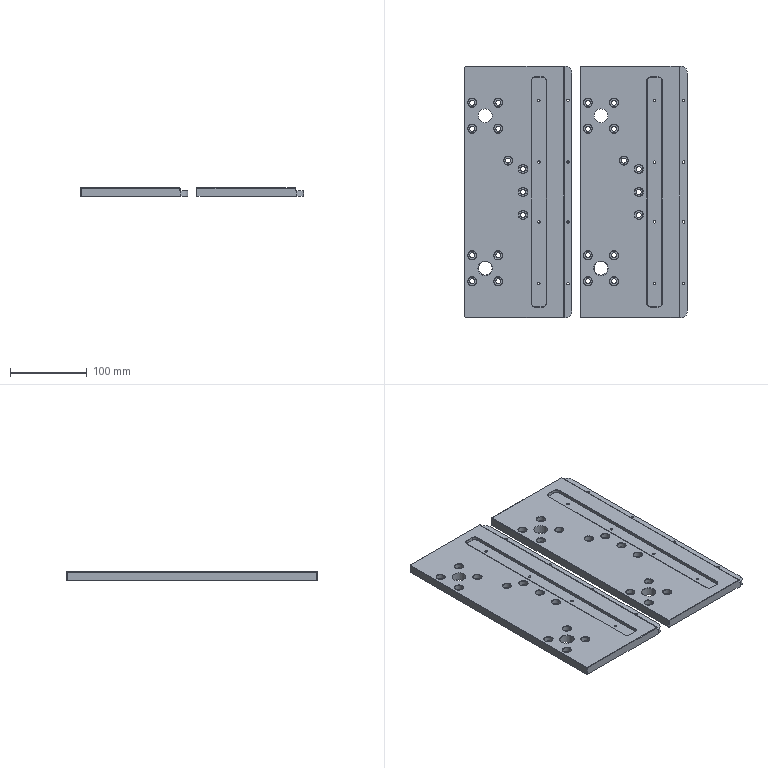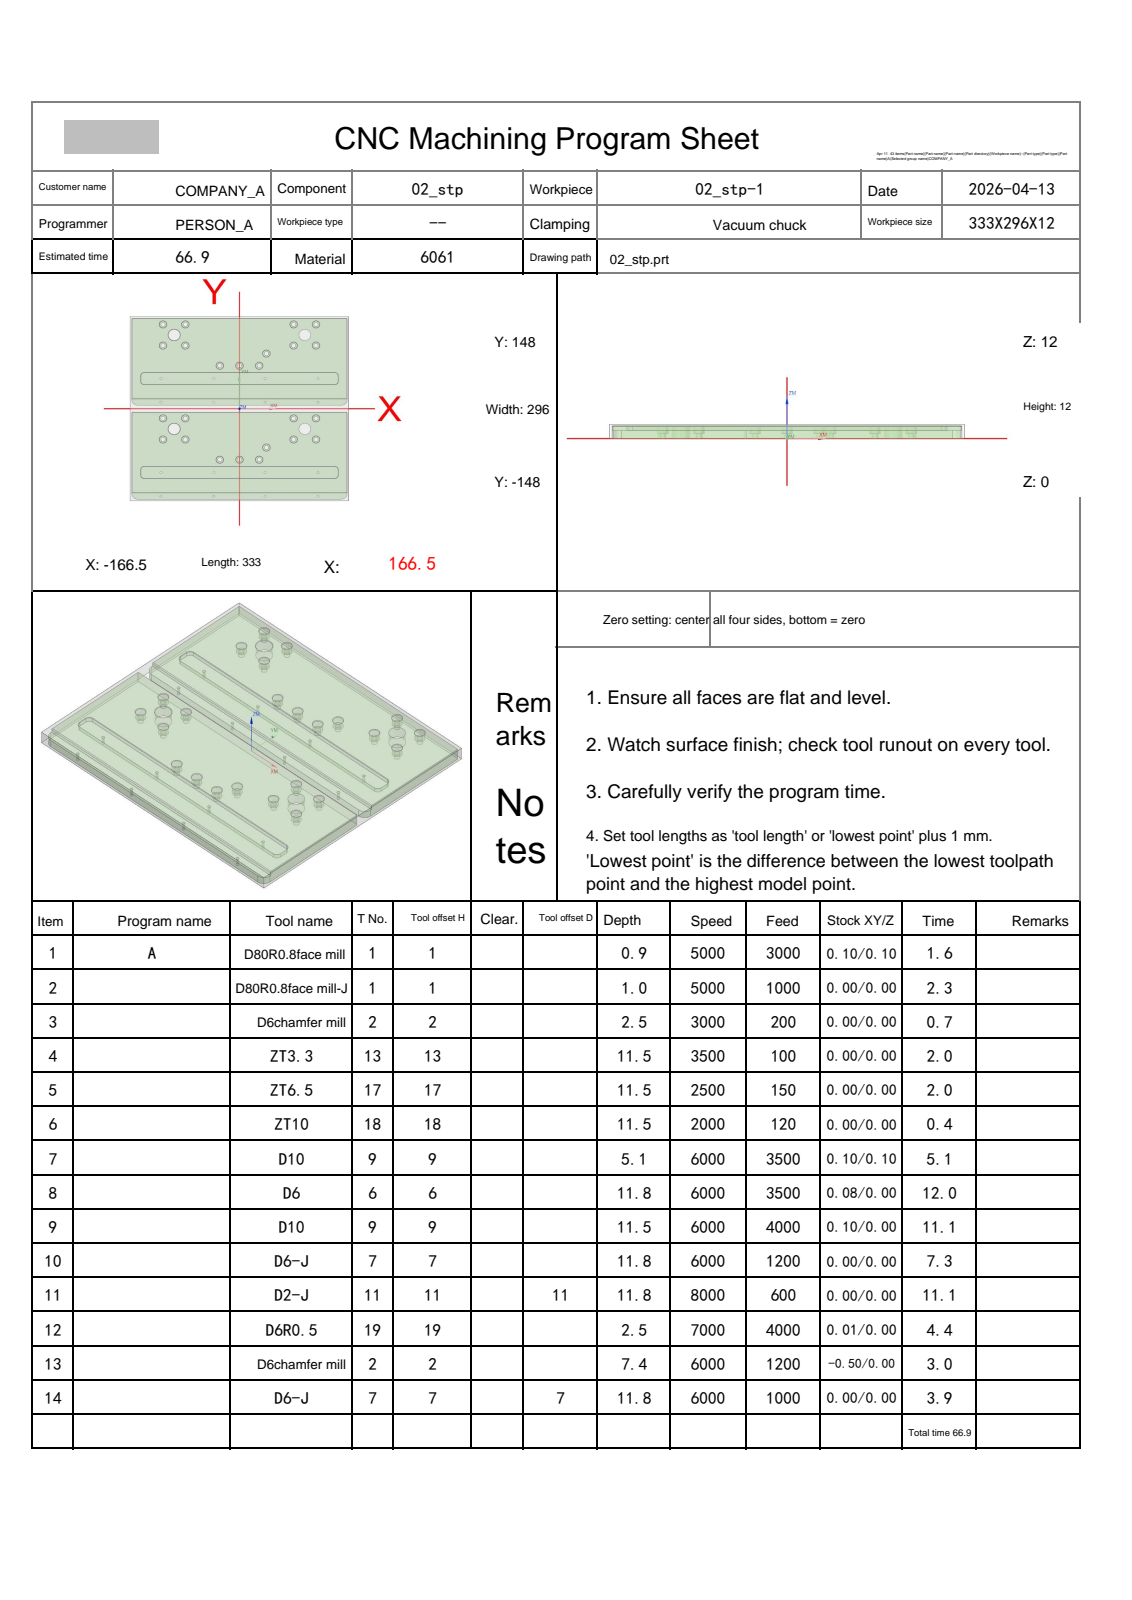NC program | NX | posted by the shop | part box 291 x 328 x 11 mm
Lines 3920 to 4804 of 9762:
N11 T11 M06
(D2-J  D=2. R=0. H=11 ce=0.00 di=0.00)
G00 G90 G54 X80.455 Y134.651 M03 S8000
G43 H11 Z31.
M08
Z5.
G01 X80.479 Y134.582 Z4.996 F600.
X80.675 Y134.236 Z4.975
X80.93 Y133.93 Z4.954
X81.236 Y133.675 Z4.934
X81.582 Y133.479 Z4.913
X81.958 Y133.347 Z4.892
X82.351 Y133.285 Z4.871
X82.649 Z4.855
X83.042 Y133.347 Z4.835
X83.418 Y133.479 Z4.814
X83.764 Y133.675 Z4.793
X84.07 Y133.93 Z4.772
X84.325 Y134.236 Z4.751
X84.521 Y134.582 Z4.73
X84.653 Y134.958 Z4.709
X84.715 Y135.351 Z4.688
Y135.649 Z4.673
X84.654 Y136.038 Z4.652
X84.525 Y136.41 Z4.632
X84.332 Y136.753 Z4.611
X84.082 Y137.057 Z4.59
X83.782 Y137.312 Z4.57
X83.442 Y137.51 Z4.549
X83.072 Y137.645 Z4.528
X82.684 Y137.712 Z4.508
X82.535 Y137.715 Z4.5
G41 D11
X82.5 Y137.75
G03 X80.25 Y135.5 Z4.417 I0.0 J-2.25
X82.5 Y133.25 Z4.335 I2.25 J0.0
X84.75 Y135.5 Z4.252 I0.0 J2.25
X82.5 Y137.75 Z4.169 I-2.25 J0.0
X80.25 Y135.5 Z4.087 I0.0 J-2.25
X82.5 Y133.25 Z4.004 I2.25 J0.0
X84.75 Y135.5 Z3.921 I0.0 J2.25
X82.5 Y137.75 Z3.838 I-2.25 J0.0
X80.25 Y135.5 Z3.756 I0.0 J-2.25
X82.5 Y133.25 Z3.673 I2.25 J0.0
X84.75 Y135.5 Z3.59 I0.0 J2.25
X82.5 Y137.75 Z3.508 I-2.25 J0.0
X80.25 Y135.5 Z3.425 I0.0 J-2.25
X82.5 Y133.25 Z3.342 I2.25 J0.0
X84.75 Y135.5 Z3.26 I0.0 J2.25
X82.5 Y137.75 Z3.177 I-2.25 J0.0
X80.25 Y135.5 Z3.094 I0.0 J-2.25
X82.5 Y133.25 Z3.012 I2.25 J0.0
X84.75 Y135.5 Z2.929 I0.0 J2.25
X82.5 Y137.75 Z2.846 I-2.25 J0.0
X80.25 Y135.5 Z2.763 I0.0 J-2.25
X82.5 Y133.25 Z2.681 I2.25 J0.0
X84.75 Y135.5 Z2.598 I0.0 J2.25
X82.5 Y137.75 Z2.515 I-2.25 J0.0
X80.25 Y135.5 Z2.433 I0.0 J-2.25
X82.5 Y133.25 Z2.35 I2.25 J0.0
X84.75 Y135.5 Z2.267 I0.0 J2.25
X82.5 Y137.75 Z2.185 I-2.25 J0.0
X80.25 Y135.5 Z2.102 I0.0 J-2.25
X82.5 Y133.25 Z2.019 I2.25 J0.0
X84.75 Y135.5 Z1.937 I0.0 J2.25
X82.5 Y137.75 Z1.854 I-2.25 J0.0
X80.25 Y135.5 Z1.771 I0.0 J-2.25
X82.5 Y133.25 Z1.688 I2.25 J0.0
X84.75 Y135.5 Z1.606 I0.0 J2.25
X82.5 Y137.75 Z1.523 I-2.25 J0.0
X80.25 Y135.5 Z1.44 I0.0 J-2.25
X82.5 Y133.25 Z1.358 I2.25 J0.0
X84.75 Y135.5 Z1.275 I0.0 J2.25
X82.5 Y137.75 Z1.192 I-2.25 J0.0
X80.25 Y135.5 Z1.11 I0.0 J-2.25
X82.5 Y133.25 Z1.027 I2.25 J0.0
X84.75 Y135.5 Z.944 I0.0 J2.25
X82.5 Y137.75 Z.862 I-2.25 J0.0
X80.25 Y135.5 Z.779 I0.0 J-2.25
X82.5 Y133.25 Z.696 I2.25 J0.0
X84.75 Y135.5 Z.613 I0.0 J2.25
X82.5 Y137.75 Z.531 I-2.25 J0.0
X80.25 Y135.5 Z.448 I0.0 J-2.25
X82.5 Y133.25 Z.365 I2.25 J0.0
X84.75 Y135.5 Z.283 I0.0 J2.25
X82.5 Y137.75 Z.2 I-2.25 J0.0
X80.25 Y135.5 I0.0 J-2.25
X82.5 Y133.25 I2.25 J0.0
X84.75 Y135.5 I0.0 J2.25
X82.5 Y137.75 I-2.25 J0.0
X82.102 Y137.715 I0.0 J-2.25
G01 X82.075 Y137.707
X82.059 Y137.684
X82.062 Y137.656
G40 X82.071 Y137.607
Z1.2
G00 Z31.
X114.455 Y134.651
Z5.
G01 X114.479 Y134.582 Z4.996
X114.675 Y134.236 Z4.975
X114.93 Y133.93 Z4.954
X115.236 Y133.675 Z4.934
X115.582 Y133.479 Z4.913
X115.958 Y133.347 Z4.892
X116.351 Y133.285 Z4.871
X116.649 Z4.855
X117.042 Y133.347 Z4.835
X117.418 Y133.479 Z4.814
X117.764 Y133.675 Z4.793
X118.07 Y133.93 Z4.772
X118.325 Y134.236 Z4.751
X118.521 Y134.582 Z4.73
X118.653 Y134.958 Z4.709
X118.715 Y135.351 Z4.688
Y135.649 Z4.673
X118.654 Y136.038 Z4.652
X118.525 Y136.41 Z4.632
X118.332 Y136.753 Z4.611
X118.082 Y137.057 Z4.59
X117.782 Y137.312 Z4.57
X117.442 Y137.51 Z4.549
X117.072 Y137.645 Z4.528
X116.684 Y137.712 Z4.508
X116.535 Y137.715 Z4.5
G41 D11
X116.5 Y137.75
G03 X114.25 Y135.5 Z4.417 I0.0 J-2.25
X116.5 Y133.25 Z4.335 I2.25 J0.0
X118.75 Y135.5 Z4.252 I0.0 J2.25
X116.5 Y137.75 Z4.169 I-2.25 J0.0
X114.25 Y135.5 Z4.087 I0.0 J-2.25
X116.5 Y133.25 Z4.004 I2.25 J0.0
X118.75 Y135.5 Z3.921 I0.0 J2.25
X116.5 Y137.75 Z3.838 I-2.25 J0.0
X114.25 Y135.5 Z3.756 I0.0 J-2.25
X116.5 Y133.25 Z3.673 I2.25 J0.0
X118.75 Y135.5 Z3.59 I0.0 J2.25
X116.5 Y137.75 Z3.508 I-2.25 J0.0
X114.25 Y135.5 Z3.425 I0.0 J-2.25
X116.5 Y133.25 Z3.342 I2.25 J0.0
X118.75 Y135.5 Z3.26 I0.0 J2.25
X116.5 Y137.75 Z3.177 I-2.25 J0.0
X114.25 Y135.5 Z3.094 I0.0 J-2.25
X116.5 Y133.25 Z3.012 I2.25 J0.0
X118.75 Y135.5 Z2.929 I0.0 J2.25
X116.5 Y137.75 Z2.846 I-2.25 J0.0
X114.25 Y135.5 Z2.763 I0.0 J-2.25
X116.5 Y133.25 Z2.681 I2.25 J0.0
X118.75 Y135.5 Z2.598 I0.0 J2.25
X116.5 Y137.75 Z2.515 I-2.25 J0.0
X114.25 Y135.5 Z2.433 I0.0 J-2.25
X116.5 Y133.25 Z2.35 I2.25 J0.0
X118.75 Y135.5 Z2.267 I0.0 J2.25
X116.5 Y137.75 Z2.185 I-2.25 J0.0
X114.25 Y135.5 Z2.102 I0.0 J-2.25
X116.5 Y133.25 Z2.019 I2.25 J0.0
X118.75 Y135.5 Z1.937 I0.0 J2.25
X116.5 Y137.75 Z1.854 I-2.25 J0.0
X114.25 Y135.5 Z1.771 I0.0 J-2.25
X116.5 Y133.25 Z1.688 I2.25 J0.0
X118.75 Y135.5 Z1.606 I0.0 J2.25
X116.5 Y137.75 Z1.523 I-2.25 J0.0
X114.25 Y135.5 Z1.44 I0.0 J-2.25
X116.5 Y133.25 Z1.358 I2.25 J0.0
X118.75 Y135.5 Z1.275 I0.0 J2.25
X116.5 Y137.75 Z1.192 I-2.25 J0.0
X114.25 Y135.5 Z1.11 I0.0 J-2.25
X116.5 Y133.25 Z1.027 I2.25 J0.0
X118.75 Y135.5 Z.944 I0.0 J2.25
X116.5 Y137.75 Z.862 I-2.25 J0.0
X114.25 Y135.5 Z.779 I0.0 J-2.25
X116.5 Y133.25 Z.696 I2.25 J0.0
X118.75 Y135.5 Z.613 I0.0 J2.25
X116.5 Y137.75 Z.531 I-2.25 J0.0
X114.25 Y135.5 Z.448 I0.0 J-2.25
X116.5 Y133.25 Z.365 I2.25 J0.0
X118.75 Y135.5 Z.283 I0.0 J2.25
X116.5 Y137.75 Z.2 I-2.25 J0.0
X114.25 Y135.5 I0.0 J-2.25
X116.5 Y133.25 I2.25 J0.0
X118.75 Y135.5 I0.0 J2.25
X116.5 Y137.75 I-2.25 J0.0
X116.102 Y137.715 I0.0 J-2.25
G01 X116.075 Y137.707
X116.059 Y137.684
X116.062 Y137.656
G40 X116.071 Y137.607
Z1.2
G00 Z31.
X114.455 Y100.651
Z5.
G01 X114.479 Y100.582 Z4.996
X114.675 Y100.236 Z4.975
X114.93 Y99.93 Z4.954
X115.236 Y99.675 Z4.934
X115.582 Y99.479 Z4.913
X115.958 Y99.347 Z4.892
X116.351 Y99.285 Z4.871
X116.649 Z4.855
X117.042 Y99.347 Z4.835
X117.418 Y99.479 Z4.814
X117.764 Y99.675 Z4.793
X118.07 Y99.93 Z4.772
X118.325 Y100.236 Z4.751
X118.521 Y100.582 Z4.73
X118.653 Y100.958 Z4.709
X118.715 Y101.351 Z4.688
Y101.649 Z4.673
X118.654 Y102.038 Z4.652
X118.525 Y102.41 Z4.632
X118.332 Y102.753 Z4.611
X118.082 Y103.057 Z4.59
X117.782 Y103.312 Z4.57
X117.442 Y103.51 Z4.549
X117.072 Y103.645 Z4.528
X116.684 Y103.712 Z4.508
X116.535 Y103.715 Z4.5
G41 D11
X116.5 Y103.75
G03 X114.884 Y103.065 Z4.458 I0.0 J-2.25
X114.25 Y101.5 Z4.417 I1.616 J-1.565
X116.5 Y99.25 Z4.335 I2.25 J0.0
X118.75 Y101.5 Z4.252 I0.0 J2.25
X116.5 Y103.75 Z4.169 I-2.25 J0.0
X114.884 Y103.065 Z4.127 I0.0 J-2.25
X114.25 Y101.5 Z4.087 I1.616 J-1.565
X116.5 Y99.25 Z4.004 I2.25 J0.0
X118.75 Y101.5 Z3.921 I0.0 J2.25
X116.5 Y103.75 Z3.838 I-2.25 J0.0
X114.884 Y103.065 Z3.796 I0.0 J-2.25
X114.25 Y101.5 Z3.756 I1.616 J-1.565
X116.5 Y99.25 Z3.673 I2.25 J0.0
X118.75 Y101.5 Z3.59 I0.0 J2.25
X116.5 Y103.75 Z3.508 I-2.25 J0.0
X114.884 Y103.065 Z3.466 I0.0 J-2.25
X114.25 Y101.5 Z3.425 I1.616 J-1.565
X116.5 Y99.25 Z3.342 I2.25 J0.0
X118.75 Y101.5 Z3.26 I0.0 J2.25
X116.5 Y103.75 Z3.177 I-2.25 J0.0
X114.884 Y103.065 Z3.135 I0.0 J-2.25
X114.25 Y101.5 Z3.094 I1.616 J-1.565
X116.5 Y99.25 Z3.012 I2.25 J0.0
X118.75 Y101.5 Z2.929 I0.0 J2.25
X116.5 Y103.75 Z2.846 I-2.25 J0.0
X114.884 Y103.065 Z2.804 I0.0 J-2.25
X114.25 Y101.5 Z2.763 I1.616 J-1.565
X116.5 Y99.25 Z2.681 I2.25 J0.0
X118.75 Y101.5 Z2.598 I0.0 J2.25
X116.5 Y103.75 Z2.515 I-2.25 J0.0
X114.884 Y103.065 Z2.473 I0.0 J-2.25
X114.25 Y101.5 Z2.433 I1.616 J-1.565
X116.5 Y99.25 Z2.35 I2.25 J0.0
X118.75 Y101.5 Z2.267 I0.0 J2.25
X116.5 Y103.75 Z2.185 I-2.25 J0.0
X114.884 Y103.065 Z2.142 I0.0 J-2.25
X114.25 Y101.5 Z2.102 I1.616 J-1.565
X116.5 Y99.25 Z2.019 I2.25 J0.0
X118.75 Y101.5 Z1.937 I0.0 J2.25
X116.5 Y103.75 Z1.854 I-2.25 J0.0
X114.884 Y103.065 Z1.812 I0.0 J-2.25
X114.25 Y101.5 Z1.771 I1.616 J-1.565
X116.5 Y99.25 Z1.688 I2.25 J0.0
X118.75 Y101.5 Z1.606 I0.0 J2.25
X116.5 Y103.75 Z1.523 I-2.25 J0.0
X114.884 Y103.065 Z1.481 I0.0 J-2.25
X114.25 Y101.5 Z1.44 I1.616 J-1.565
X116.5 Y99.25 Z1.358 I2.25 J0.0
X118.75 Y101.5 Z1.275 I0.0 J2.25
X116.5 Y103.75 Z1.192 I-2.25 J0.0
X114.884 Y103.065 Z1.15 I0.0 J-2.25
X114.25 Y101.5 Z1.11 I1.616 J-1.565
X116.5 Y99.25 Z1.027 I2.25 J0.0
X118.75 Y101.5 Z.944 I0.0 J2.25
X116.5 Y103.75 Z.862 I-2.25 J0.0
X114.884 Y103.065 Z.819 I0.0 J-2.25
X114.25 Y101.5 Z.779 I1.616 J-1.565
X116.5 Y99.25 Z.696 I2.25 J0.0
X118.75 Y101.5 Z.613 I0.0 J2.25
X116.5 Y103.75 Z.531 I-2.25 J0.0
X114.884 Y103.065 Z.489 I0.0 J-2.25
X114.25 Y101.5 Z.448 I1.616 J-1.565
X116.5 Y99.25 Z.365 I2.25 J0.0
X118.75 Y101.5 Z.283 I0.0 J2.25
X116.5 Y103.75 Z.2 I-2.25 J0.0
X114.25 Y101.5 I0.0 J-2.25
X116.5 Y99.25 I2.25 J0.0
X118.75 Y101.5 I0.0 J2.25
X116.5 Y103.75 I-2.25 J0.0
X116.102 Y103.715 I0.0 J-2.25
G01 X116.075 Y103.707
X116.059 Y103.684
X116.062 Y103.656
G40 X116.071 Y103.607
Z1.2
G00 Z31.
X80.455 Y100.651
Z5.
G01 X80.479 Y100.582 Z4.996
X80.675 Y100.236 Z4.975
X80.93 Y99.93 Z4.954
X81.236 Y99.675 Z4.934
X81.582 Y99.479 Z4.913
X81.958 Y99.347 Z4.892
X82.351 Y99.285 Z4.871
X82.649 Z4.855
X83.042 Y99.347 Z4.835
X83.418 Y99.479 Z4.814
X83.764 Y99.675 Z4.793
X84.07 Y99.93 Z4.772
X84.325 Y100.236 Z4.751
X84.521 Y100.582 Z4.73
X84.653 Y100.958 Z4.709
X84.715 Y101.351 Z4.688
Y101.649 Z4.673
X84.654 Y102.038 Z4.652
X84.525 Y102.41 Z4.632
X84.332 Y102.753 Z4.611
X84.082 Y103.057 Z4.59
X83.782 Y103.312 Z4.57
X83.442 Y103.51 Z4.549
X83.072 Y103.645 Z4.528
X82.684 Y103.712 Z4.508
X82.535 Y103.715 Z4.5
G41 D11
X82.5 Y103.75
G03 X80.25 Y101.5 Z4.417 I0.0 J-2.25
X82.5 Y99.25 Z4.335 I2.25 J0.0
X84.75 Y101.5 Z4.252 I0.0 J2.25
X82.5 Y103.75 Z4.169 I-2.25 J0.0
X80.25 Y101.5 Z4.087 I0.0 J-2.25
X82.5 Y99.25 Z4.004 I2.25 J0.0
X84.75 Y101.5 Z3.921 I0.0 J2.25
X82.5 Y103.75 Z3.838 I-2.25 J0.0
X80.25 Y101.5 Z3.756 I0.0 J-2.25
X82.5 Y99.25 Z3.673 I2.25 J0.0
X84.75 Y101.5 Z3.59 I0.0 J2.25
X82.5 Y103.75 Z3.508 I-2.25 J0.0
X80.25 Y101.5 Z3.425 I0.0 J-2.25
X82.5 Y99.25 Z3.342 I2.25 J0.0
X84.75 Y101.5 Z3.26 I0.0 J2.25
X82.5 Y103.75 Z3.177 I-2.25 J0.0
X80.25 Y101.5 Z3.094 I0.0 J-2.25
X82.5 Y99.25 Z3.012 I2.25 J0.0
X84.75 Y101.5 Z2.929 I0.0 J2.25
X82.5 Y103.75 Z2.846 I-2.25 J0.0
X80.25 Y101.5 Z2.763 I0.0 J-2.25
X82.5 Y99.25 Z2.681 I2.25 J0.0
X84.75 Y101.5 Z2.598 I0.0 J2.25
X82.5 Y103.75 Z2.515 I-2.25 J0.0
X80.25 Y101.5 Z2.433 I0.0 J-2.25
X82.5 Y99.25 Z2.35 I2.25 J0.0
X84.75 Y101.5 Z2.267 I0.0 J2.25
X82.5 Y103.75 Z2.185 I-2.25 J0.0
X80.25 Y101.5 Z2.102 I0.0 J-2.25
X82.5 Y99.25 Z2.019 I2.25 J0.0
X84.75 Y101.5 Z1.937 I0.0 J2.25
X82.5 Y103.75 Z1.854 I-2.25 J0.0
X80.25 Y101.5 Z1.771 I0.0 J-2.25
X82.5 Y99.25 Z1.688 I2.25 J0.0
X84.75 Y101.5 Z1.606 I0.0 J2.25
X82.5 Y103.75 Z1.523 I-2.25 J0.0
X80.25 Y101.5 Z1.44 I0.0 J-2.25
X82.5 Y99.25 Z1.358 I2.25 J0.0
X84.75 Y101.5 Z1.275 I0.0 J2.25
X82.5 Y103.75 Z1.192 I-2.25 J0.0
X80.25 Y101.5 Z1.11 I0.0 J-2.25
X82.5 Y99.25 Z1.027 I2.25 J0.0
X84.75 Y101.5 Z.944 I0.0 J2.25
X82.5 Y103.75 Z.862 I-2.25 J0.0
X80.25 Y101.5 Z.779 I0.0 J-2.25
X82.5 Y99.25 Z.696 I2.25 J0.0
X84.75 Y101.5 Z.613 I0.0 J2.25
X82.5 Y103.75 Z.531 I-2.25 J0.0
X80.25 Y101.5 Z.448 I0.0 J-2.25
X82.5 Y99.25 Z.365 I2.25 J0.0
X84.75 Y101.5 Z.283 I0.0 J2.25
X82.5 Y103.75 Z.2 I-2.25 J0.0
X80.25 Y101.5 I0.0 J-2.25
X82.5 Y99.25 I2.25 J0.0
X84.75 Y101.5 I0.0 J2.25
X82.5 Y103.75 I-2.25 J0.0
X82.102 Y103.715 I0.0 J-2.25
G01 X82.075 Y103.707
X82.059 Y103.684
X82.062 Y103.656
G40 X82.071 Y103.607
Z1.2
G00 Z31.
X38.955 Y87.751
Z5.
G01 X38.979 Y87.682 Z4.996
X39.175 Y87.336 Z4.975
X39.43 Y87.03 Z4.954
X39.736 Y86.775 Z4.934
X40.082 Y86.579 Z4.913
X40.458 Y86.447 Z4.892
X40.851 Y86.385 Z4.871
X41.149 Z4.855
X41.542 Y86.447 Z4.835
X41.918 Y86.579 Z4.814
X42.264 Y86.775 Z4.793
X42.57 Y87.03 Z4.772
X42.825 Y87.336 Z4.751
X43.021 Y87.682 Z4.73
X43.153 Y88.058 Z4.709
X43.215 Y88.451 Z4.688
Y88.749 Z4.673
X43.154 Y89.138 Z4.652
X43.025 Y89.51 Z4.632
X42.832 Y89.853 Z4.611
X42.582 Y90.157 Z4.59
X42.282 Y90.412 Z4.57
X41.942 Y90.61 Z4.549
X41.572 Y90.745 Z4.528
X41.184 Y90.812 Z4.508
X41.035 Y90.815 Z4.5
G41 D11
X41. Y90.85
G03 X38.75 Y88.6 Z4.417 I0.0 J-2.25
X41. Y86.35 Z4.335 I2.25 J0.0
X43.25 Y88.6 Z4.252 I0.0 J2.25
X41. Y90.85 Z4.169 I-2.25 J0.0
X38.75 Y88.6 Z4.087 I0.0 J-2.25
X41. Y86.35 Z4.004 I2.25 J0.0
X43.25 Y88.6 Z3.921 I0.0 J2.25
X41. Y90.85 Z3.838 I-2.25 J0.0
X38.75 Y88.6 Z3.756 I0.0 J-2.25
X41. Y86.35 Z3.673 I2.25 J0.0
X43.25 Y88.6 Z3.59 I0.0 J2.25
X41. Y90.85 Z3.508 I-2.25 J0.0
X38.75 Y88.6 Z3.425 I0.0 J-2.25
X41. Y86.35 Z3.342 I2.25 J0.0
X43.25 Y88.6 Z3.26 I0.0 J2.25
X41. Y90.85 Z3.177 I-2.25 J0.0
X38.75 Y88.6 Z3.094 I0.0 J-2.25
X41. Y86.35 Z3.012 I2.25 J0.0
X43.25 Y88.6 Z2.929 I0.0 J2.25
X41. Y90.85 Z2.846 I-2.25 J0.0
X38.75 Y88.6 Z2.763 I0.0 J-2.25
X41. Y86.35 Z2.681 I2.25 J0.0
X43.25 Y88.6 Z2.598 I0.0 J2.25
X41. Y90.85 Z2.515 I-2.25 J0.0
X38.75 Y88.6 Z2.433 I0.0 J-2.25
X41. Y86.35 Z2.35 I2.25 J0.0
X43.25 Y88.6 Z2.267 I0.0 J2.25
X41. Y90.85 Z2.185 I-2.25 J0.0
X38.75 Y88.6 Z2.102 I0.0 J-2.25
X41. Y86.35 Z2.019 I2.25 J0.0
X43.25 Y88.6 Z1.937 I0.0 J2.25
X41. Y90.85 Z1.854 I-2.25 J0.0
X38.75 Y88.6 Z1.771 I0.0 J-2.25
X41. Y86.35 Z1.688 I2.25 J0.0
X43.25 Y88.6 Z1.606 I0.0 J2.25
X41. Y90.85 Z1.523 I-2.25 J0.0
X38.75 Y88.6 Z1.44 I0.0 J-2.25
X41. Y86.35 Z1.358 I2.25 J0.0
X43.25 Y88.6 Z1.275 I0.0 J2.25
X41. Y90.85 Z1.192 I-2.25 J0.0
X38.75 Y88.6 Z1.11 I0.0 J-2.25
X41. Y86.35 Z1.027 I2.25 J0.0
X43.25 Y88.6 Z.944 I0.0 J2.25
X41. Y90.85 Z.862 I-2.25 J0.0
X38.75 Y88.6 Z.779 I0.0 J-2.25
X41. Y86.35 Z.696 I2.25 J0.0
X43.25 Y88.6 Z.613 I0.0 J2.25
X41. Y90.85 Z.531 I-2.25 J0.0
X38.75 Y88.6 Z.448 I0.0 J-2.25
X41. Y86.35 Z.365 I2.25 J0.0
X43.25 Y88.6 Z.283 I0.0 J2.25
X41. Y90.85 Z.2 I-2.25 J0.0
X38.75 Y88.6 I0.0 J-2.25
X41. Y86.35 I2.25 J0.0
X43.25 Y88.6 I0.0 J2.25
X41. Y90.85 I-2.25 J0.0
X40.602 Y90.815 I0.0 J-2.25
G01 X40.575 Y90.807
X40.559 Y90.784
X40.562 Y90.756
G40 X40.571 Y90.707
Z1.2
G00 Z31.
X28.005 Y68.251
Z5.
G01 X28.029 Y68.182 Z4.996
X28.225 Y67.836 Z4.975
X28.48 Y67.53 Z4.954
X28.786 Y67.275 Z4.934
X29.132 Y67.079 Z4.913
X29.508 Y66.947 Z4.892
X29.901 Y66.885 Z4.871
X30.199 Z4.855
X30.592 Y66.947 Z4.835
X30.968 Y67.079 Z4.814
X31.314 Y67.275 Z4.793
X31.62 Y67.53 Z4.772
X31.875 Y67.836 Z4.751
X32.071 Y68.182 Z4.73
X32.203 Y68.558 Z4.709
X32.265 Y68.951 Z4.688
Y69.249 Z4.673
X32.204 Y69.638 Z4.652
X32.075 Y70.01 Z4.632
X31.882 Y70.353 Z4.611
X31.632 Y70.657 Z4.59
X31.332 Y70.912 Z4.57
X30.992 Y71.11 Z4.549
X30.622 Y71.245 Z4.528
X30.234 Y71.312 Z4.508
X30.085 Y71.315 Z4.5
G41 D11
X30.05 Y71.35
G03 X27.8 Y69.1 Z4.417 I0.0 J-2.25
X30.05 Y66.85 Z4.335 I2.25 J0.0
X32.3 Y69.1 Z4.252 I0.0 J2.25
X30.05 Y71.35 Z4.169 I-2.25 J0.0
X27.8 Y69.1 Z4.087 I0.0 J-2.25
X30.05 Y66.85 Z4.004 I2.25 J0.0
X32.3 Y69.1 Z3.921 I0.0 J2.25
X30.05 Y71.35 Z3.838 I-2.25 J0.0
X27.8 Y69.1 Z3.756 I0.0 J-2.25
X30.05 Y66.85 Z3.673 I2.25 J0.0
X32.3 Y69.1 Z3.59 I0.0 J2.25
X30.05 Y71.35 Z3.508 I-2.25 J0.0
X27.8 Y69.1 Z3.425 I0.0 J-2.25
X30.05 Y66.85 Z3.342 I2.25 J0.0
X32.3 Y69.1 Z3.26 I0.0 J2.25
X30.05 Y71.35 Z3.177 I-2.25 J0.0
X27.8 Y69.1 Z3.094 I0.0 J-2.25
X30.05 Y66.85 Z3.012 I2.25 J0.0
X32.3 Y69.1 Z2.929 I0.0 J2.25
X30.05 Y71.35 Z2.846 I-2.25 J0.0
X27.8 Y69.1 Z2.763 I0.0 J-2.25
X30.05 Y66.85 Z2.681 I2.25 J0.0
X32.3 Y69.1 Z2.598 I0.0 J2.25
X30.05 Y71.35 Z2.515 I-2.25 J0.0
X27.8 Y69.1 Z2.433 I0.0 J-2.25
X30.05 Y66.85 Z2.35 I2.25 J0.0
X32.3 Y69.1 Z2.267 I0.0 J2.25
X30.05 Y71.35 Z2.185 I-2.25 J0.0
X27.8 Y69.1 Z2.102 I0.0 J-2.25
X30.05 Y66.85 Z2.019 I2.25 J0.0
X32.3 Y69.1 Z1.937 I0.0 J2.25
X30.05 Y71.35 Z1.854 I-2.25 J0.0
X27.8 Y69.1 Z1.771 I0.0 J-2.25
X30.05 Y66.85 Z1.688 I2.25 J0.0
X32.3 Y69.1 Z1.606 I0.0 J2.25
X30.05 Y71.35 Z1.523 I-2.25 J0.0
X27.8 Y69.1 Z1.44 I0.0 J-2.25
X30.05 Y66.85 Z1.358 I2.25 J0.0
X32.3 Y69.1 Z1.275 I0.0 J2.25
X30.05 Y71.35 Z1.192 I-2.25 J0.0
X27.8 Y69.1 Z1.11 I0.0 J-2.25
X30.05 Y66.85 Z1.027 I2.25 J0.0
X32.3 Y69.1 Z.944 I0.0 J2.25
X30.05 Y71.35 Z.862 I-2.25 J0.0
X27.8 Y69.1 Z.779 I0.0 J-2.25
X30.05 Y66.85 Z.696 I2.25 J0.0
X32.3 Y69.1 Z.613 I0.0 J2.25
X30.05 Y71.35 Z.531 I-2.25 J0.0
X27.8 Y69.1 Z.448 I0.0 J-2.25
X30.05 Y66.85 Z.365 I2.25 J0.0
X32.3 Y69.1 Z.283 I0.0 J2.25
X30.05 Y71.35 Z.2 I-2.25 J0.0
X27.8 Y69.1 I0.0 J-2.25
X30.05 Y66.85 I2.25 J0.0
X32.3 Y69.1 I0.0 J2.25
X30.05 Y71.35 I-2.25 J0.0
X29.652 Y71.315 I0.0 J-2.25
G01 X29.625 Y71.307
X29.609 Y71.284
X29.612 Y71.256
G40 X29.621 Y71.207
Z1.2
G00 Z31.
X-1.995 Y68.251
Z5.
G01 X-1.971 Y68.182 Z4.996
X-1.775 Y67.836 Z4.975
X-1.52 Y67.53 Z4.954
X-1.214 Y67.275 Z4.934
X-.868 Y67.079 Z4.913
X-.492 Y66.947 Z4.892
X-.099 Y66.885 Z4.871
X.199 Z4.855
X.592 Y66.947 Z4.835
X.968 Y67.079 Z4.814
X1.314 Y67.275 Z4.793
X1.62 Y67.53 Z4.772
X1.875 Y67.836 Z4.751
X2.071 Y68.182 Z4.73
X2.203 Y68.558 Z4.709
X2.265 Y68.951 Z4.688
Y69.249 Z4.673
X2.204 Y69.638 Z4.652
X2.075 Y70.01 Z4.632
X1.882 Y70.353 Z4.611
X1.632 Y70.657 Z4.59
X1.332 Y70.912 Z4.57
X.992 Y71.11 Z4.549
X.622 Y71.245 Z4.528
X.234 Y71.312 Z4.508
X.085 Y71.315 Z4.5
G41 D11
X.05 Y71.35
G03 X-2.2 Y69.1 Z4.417 I0.0 J-2.25
X.05 Y66.85 Z4.335 I2.25 J0.0
X2.3 Y69.1 Z4.252 I0.0 J2.25
X.05 Y71.35 Z4.169 I-2.25 J0.0
X-2.2 Y69.1 Z4.087 I0.0 J-2.25
X.05 Y66.85 Z4.004 I2.25 J0.0
X2.3 Y69.1 Z3.921 I0.0 J2.25
X.05 Y71.35 Z3.838 I-2.25 J0.0
X-2.2 Y69.1 Z3.756 I0.0 J-2.25
X.05 Y66.85 Z3.673 I2.25 J0.0
X2.3 Y69.1 Z3.59 I0.0 J2.25
X.05 Y71.35 Z3.508 I-2.25 J0.0
X-2.2 Y69.1 Z3.425 I0.0 J-2.25
X.05 Y66.85 Z3.342 I2.25 J0.0
X2.3 Y69.1 Z3.26 I0.0 J2.25
X.05 Y71.35 Z3.177 I-2.25 J0.0
X-2.2 Y69.1 Z3.094 I0.0 J-2.25
X.05 Y66.85 Z3.012 I2.25 J0.0
X2.3 Y69.1 Z2.929 I0.0 J2.25
X.05 Y71.35 Z2.846 I-2.25 J0.0
X-2.2 Y69.1 Z2.763 I0.0 J-2.25
X.05 Y66.85 Z2.681 I2.25 J0.0
X2.3 Y69.1 Z2.598 I0.0 J2.25
X.05 Y71.35 Z2.515 I-2.25 J0.0
X-2.2 Y69.1 Z2.433 I0.0 J-2.25
X.05 Y66.85 Z2.35 I2.25 J0.0
X2.3 Y69.1 Z2.267 I0.0 J2.25
X.05 Y71.35 Z2.185 I-2.25 J0.0
X-2.2 Y69.1 Z2.102 I0.0 J-2.25
X.05 Y66.85 Z2.019 I2.25 J0.0
X2.3 Y69.1 Z1.937 I0.0 J2.25
X.05 Y71.35 Z1.854 I-2.25 J0.0
X-2.2 Y69.1 Z1.771 I0.0 J-2.25
X.05 Y66.85 Z1.688 I2.25 J0.0
X2.3 Y69.1 Z1.606 I0.0 J2.25
X.05 Y71.35 Z1.523 I-2.25 J0.0
X-2.2 Y69.1 Z1.44 I0.0 J-2.25
X.05 Y66.85 Z1.358 I2.25 J0.0
X2.3 Y69.1 Z1.275 I0.0 J2.25
X.05 Y71.35 Z1.192 I-2.25 J0.0
X-2.2 Y69.1 Z1.11 I0.0 J-2.25
X.05 Y66.85 Z1.027 I2.25 J0.0
X2.3 Y69.1 Z.944 I0.0 J2.25
X.05 Y71.35 Z.862 I-2.25 J0.0
X-2.2 Y69.1 Z.779 I0.0 J-2.25
X.05 Y66.85 Z.696 I2.25 J0.0
X2.3 Y69.1 Z.613 I0.0 J2.25
X.05 Y71.35 Z.531 I-2.25 J0.0
X-2.2 Y69.1 Z.448 I0.0 J-2.25
X.05 Y66.85 Z.365 I2.25 J0.0
X2.3 Y69.1 Z.283 I0.0 J2.25
X.05 Y71.35 Z.2 I-2.25 J0.0
X-2.2 Y69.1 I0.0 J-2.25
X.05 Y66.85 I2.25 J0.0
X2.3 Y69.1 I0.0 J2.25
X.05 Y71.35 I-2.25 J0.0
X-.348 Y71.315 I0.0 J-2.25
G01 X-.375 Y71.307
X-.391 Y71.284
X-.388 Y71.256
G40 X-.379 Y71.207
Z1.2
G00 Z31.
X-31.995 Y68.251
Z5.
G01 X-31.971 Y68.182 Z4.996
X-31.775 Y67.836 Z4.975
X-31.52 Y67.53 Z4.954
X-31.214 Y67.275 Z4.934
X-30.868 Y67.079 Z4.913
X-30.492 Y66.947 Z4.892
X-30.099 Y66.885 Z4.871
X-29.801 Z4.855
X-29.408 Y66.947 Z4.835
X-29.032 Y67.079 Z4.814
X-28.686 Y67.275 Z4.793
X-28.38 Y67.53 Z4.772
X-28.125 Y67.836 Z4.751
X-27.929 Y68.182 Z4.73
X-27.797 Y68.558 Z4.709
X-27.735 Y68.951 Z4.688
Y69.249 Z4.673
X-27.796 Y69.638 Z4.652
X-27.925 Y70.01 Z4.632
X-28.118 Y70.353 Z4.611
X-28.368 Y70.657 Z4.59
X-28.668 Y70.912 Z4.57
X-29.008 Y71.11 Z4.549
X-29.378 Y71.245 Z4.528
X-29.766 Y71.312 Z4.508
X-29.915 Y71.315 Z4.5
G41 D11
X-29.95 Y71.35
G03 X-32.2 Y69.1 Z4.417 I0.0 J-2.25
X-29.95 Y66.85 Z4.335 I2.25 J0.0
X-27.7 Y69.1 Z4.252 I0.0 J2.25
X-29.95 Y71.35 Z4.169 I-2.25 J0.0
X-32.2 Y69.1 Z4.087 I0.0 J-2.25
X-29.95 Y66.85 Z4.004 I2.25 J0.0
X-27.7 Y69.1 Z3.921 I0.0 J2.25
X-29.95 Y71.35 Z3.838 I-2.25 J0.0
X-32.2 Y69.1 Z3.756 I0.0 J-2.25
X-29.95 Y66.85 Z3.673 I2.25 J0.0
X-27.7 Y69.1 Z3.59 I0.0 J2.25
X-29.95 Y71.35 Z3.508 I-2.25 J0.0
X-32.2 Y69.1 Z3.425 I0.0 J-2.25
X-29.95 Y66.85 Z3.342 I2.25 J0.0
X-27.7 Y69.1 Z3.26 I0.0 J2.25
X-29.95 Y71.35 Z3.177 I-2.25 J0.0
X-32.2 Y69.1 Z3.094 I0.0 J-2.25
X-29.95 Y66.85 Z3.012 I2.25 J0.0
X-27.7 Y69.1 Z2.929 I0.0 J2.25
X-29.95 Y71.35 Z2.846 I-2.25 J0.0
X-32.2 Y69.1 Z2.763 I0.0 J-2.25
X-29.95 Y66.85 Z2.681 I2.25 J0.0
X-27.7 Y69.1 Z2.598 I0.0 J2.25
X-29.95 Y71.35 Z2.515 I-2.25 J0.0
X-32.2 Y69.1 Z2.433 I0.0 J-2.25
X-29.95 Y66.85 Z2.35 I2.25 J0.0
X-27.7 Y69.1 Z2.267 I0.0 J2.25
X-29.95 Y71.35 Z2.185 I-2.25 J0.0
X-32.2 Y69.1 Z2.102 I0.0 J-2.25
X-29.95 Y66.85 Z2.019 I2.25 J0.0
X-27.7 Y69.1 Z1.937 I0.0 J2.25
X-29.95 Y71.35 Z1.854 I-2.25 J0.0
X-32.2 Y69.1 Z1.771 I0.0 J-2.25
X-29.95 Y66.85 Z1.688 I2.25 J0.0
X-27.7 Y69.1 Z1.606 I0.0 J2.25
X-29.95 Y71.35 Z1.523 I-2.25 J0.0
X-32.2 Y69.1 Z1.44 I0.0 J-2.25
X-29.95 Y66.85 Z1.358 I2.25 J0.0
X-27.7 Y69.1 Z1.275 I0.0 J2.25
X-29.95 Y71.35 Z1.192 I-2.25 J0.0
X-32.2 Y69.1 Z1.11 I0.0 J-2.25
X-29.95 Y66.85 Z1.027 I2.25 J0.0
X-27.7 Y69.1 Z.944 I0.0 J2.25
X-29.95 Y71.35 Z.862 I-2.25 J0.0
X-32.2 Y69.1 Z.779 I0.0 J-2.25
X-29.95 Y66.85 Z.696 I2.25 J0.0
X-27.7 Y69.1 Z.613 I0.0 J2.25
X-29.95 Y71.35 Z.531 I-2.25 J0.0
X-32.2 Y69.1 Z.448 I0.0 J-2.25
X-29.95 Y66.85 Z.365 I2.25 J0.0
X-27.7 Y69.1 Z.283 I0.0 J2.25
X-29.95 Y71.35 Z.2 I-2.25 J0.0
X-32.2 Y69.1 I0.0 J-2.25
X-29.95 Y66.85 I2.25 J0.0
X-27.7 Y69.1 I0.0 J2.25
X-29.95 Y71.35 I-2.25 J0.0
X-30.348 Y71.315 I0.0 J-2.25
G01 X-30.375 Y71.307
X-30.391 Y71.284
X-30.388 Y71.256
G40 X-30.379 Y71.207
Z1.2
G00 Z31.
X-84.545 Y100.651
Z5.
G01 X-84.521 Y100.582 Z4.996
X-84.325 Y100.236 Z4.975
X-84.07 Y99.93 Z4.954
X-83.764 Y99.675 Z4.934
X-83.418 Y99.479 Z4.913
X-83.042 Y99.347 Z4.892
X-82.649 Y99.285 Z4.871
X-82.351 Z4.855
X-81.958 Y99.347 Z4.835
X-81.582 Y99.479 Z4.814
X-81.236 Y99.675 Z4.793
X-80.93 Y99.93 Z4.772
X-80.675 Y100.236 Z4.751
X-80.479 Y100.582 Z4.73
X-80.347 Y100.958 Z4.709
X-80.285 Y101.351 Z4.688
Y101.649 Z4.673
X-80.346 Y102.038 Z4.652
X-80.475 Y102.41 Z4.632
X-80.668 Y102.753 Z4.611
X-80.918 Y103.057 Z4.59
X-81.218 Y103.312 Z4.57
X-81.558 Y103.51 Z4.549
X-81.928 Y103.645 Z4.528
X-82.316 Y103.712 Z4.508
X-82.465 Y103.715 Z4.5
G41 D11
X-82.5 Y103.75
G03 X-84.75 Y101.5 Z4.417 I0.0 J-2.25
X-82.5 Y99.25 Z4.335 I2.25 J0.0
X-80.25 Y101.5 Z4.252 I0.0 J2.25
X-82.5 Y103.75 Z4.169 I-2.25 J0.0
X-84.75 Y101.5 Z4.087 I0.0 J-2.25
X-82.5 Y99.25 Z4.004 I2.25 J0.0
X-80.25 Y101.5 Z3.921 I0.0 J2.25
X-82.5 Y103.75 Z3.838 I-2.25 J0.0
X-84.75 Y101.5 Z3.756 I0.0 J-2.25
X-82.5 Y99.25 Z3.673 I2.25 J0.0
X-80.25 Y101.5 Z3.59 I0.0 J2.25
X-82.5 Y103.75 Z3.508 I-2.25 J0.0
X-84.75 Y101.5 Z3.425 I0.0 J-2.25
X-82.5 Y99.25 Z3.342 I2.25 J0.0
X-80.25 Y101.5 Z3.26 I0.0 J2.25
X-82.5 Y103.75 Z3.177 I-2.25 J0.0
X-84.75 Y101.5 Z3.094 I0.0 J-2.25
X-82.5 Y99.25 Z3.012 I2.25 J0.0
X-80.25 Y101.5 Z2.929 I0.0 J2.25
X-82.5 Y103.75 Z2.846 I-2.25 J0.0
X-84.75 Y101.5 Z2.763 I0.0 J-2.25
X-82.5 Y99.25 Z2.681 I2.25 J0.0
X-80.25 Y101.5 Z2.598 I0.0 J2.25
X-82.5 Y103.75 Z2.515 I-2.25 J0.0
X-84.75 Y101.5 Z2.433 I0.0 J-2.25
X-82.5 Y99.25 Z2.35 I2.25 J0.0
X-80.25 Y101.5 Z2.267 I0.0 J2.25
X-82.5 Y103.75 Z2.185 I-2.25 J0.0
X-84.75 Y101.5 Z2.102 I0.0 J-2.25
X-82.5 Y99.25 Z2.019 I2.25 J0.0
X-80.25 Y101.5 Z1.937 I0.0 J2.25
X-82.5 Y103.75 Z1.854 I-2.25 J0.0
X-84.75 Y101.5 Z1.771 I0.0 J-2.25
X-82.5 Y99.25 Z1.688 I2.25 J0.0
X-80.25 Y101.5 Z1.606 I0.0 J2.25
X-82.5 Y103.75 Z1.523 I-2.25 J0.0
X-84.75 Y101.5 Z1.44 I0.0 J-2.25
X-82.5 Y99.25 Z1.358 I2.25 J0.0
X-80.25 Y101.5 Z1.275 I0.0 J2.25
X-82.5 Y103.75 Z1.192 I-2.25 J0.0
X-84.75 Y101.5 Z1.11 I0.0 J-2.25
X-82.5 Y99.25 Z1.027 I2.25 J0.0
X-80.25 Y101.5 Z.944 I0.0 J2.25
X-82.5 Y103.75 Z.862 I-2.25 J0.0
X-84.75 Y101.5 Z.779 I0.0 J-2.25
X-82.5 Y99.25 Z.696 I2.25 J0.0
X-80.25 Y101.5 Z.613 I0.0 J2.25
X-82.5 Y103.75 Z.531 I-2.25 J0.0
X-84.75 Y101.5 Z.448 I0.0 J-2.25
X-82.5 Y99.25 Z.365 I2.25 J0.0
X-80.25 Y101.5 Z.283 I0.0 J2.25
X-82.5 Y103.75 Z.2 I-2.25 J0.0
X-84.75 Y101.5 I0.0 J-2.25
X-82.5 Y99.25 I2.25 J0.0
X-80.25 Y101.5 I0.0 J2.25
X-82.5 Y103.75 I-2.25 J0.0
X-82.898 Y103.715 I0.0 J-2.25
G01 X-82.925 Y103.707
X-82.941 Y103.684
X-82.938 Y103.656
G40 X-82.929 Y103.607
Z1.2
G00 Z31.
X-84.545 Y134.651
Z5.
G01 X-84.521 Y134.582 Z4.996
X-84.325 Y134.236 Z4.975
X-84.07 Y133.93 Z4.954
X-83.764 Y133.675 Z4.934
X-83.418 Y133.479 Z4.913
X-83.042 Y133.347 Z4.892
X-82.649 Y133.285 Z4.871
X-82.351 Z4.855
X-81.958 Y133.347 Z4.835
X-81.582 Y133.479 Z4.814
X-81.236 Y133.675 Z4.793
X-80.93 Y133.93 Z4.772
X-80.675 Y134.236 Z4.751
X-80.479 Y134.582 Z4.73
X-80.347 Y134.958 Z4.709
X-80.285 Y135.351 Z4.688
Y135.649 Z4.673
X-80.346 Y136.038 Z4.652
X-80.475 Y136.41 Z4.632
X-80.668 Y136.753 Z4.611
X-80.918 Y137.057 Z4.59
X-81.218 Y137.312 Z4.57
X-81.558 Y137.51 Z4.549
X-81.928 Y137.645 Z4.528
X-82.316 Y137.712 Z4.508
X-82.465 Y137.715 Z4.5
G41 D11
X-82.5 Y137.75
G03 X-84.75 Y135.5 Z4.417 I0.0 J-2.25